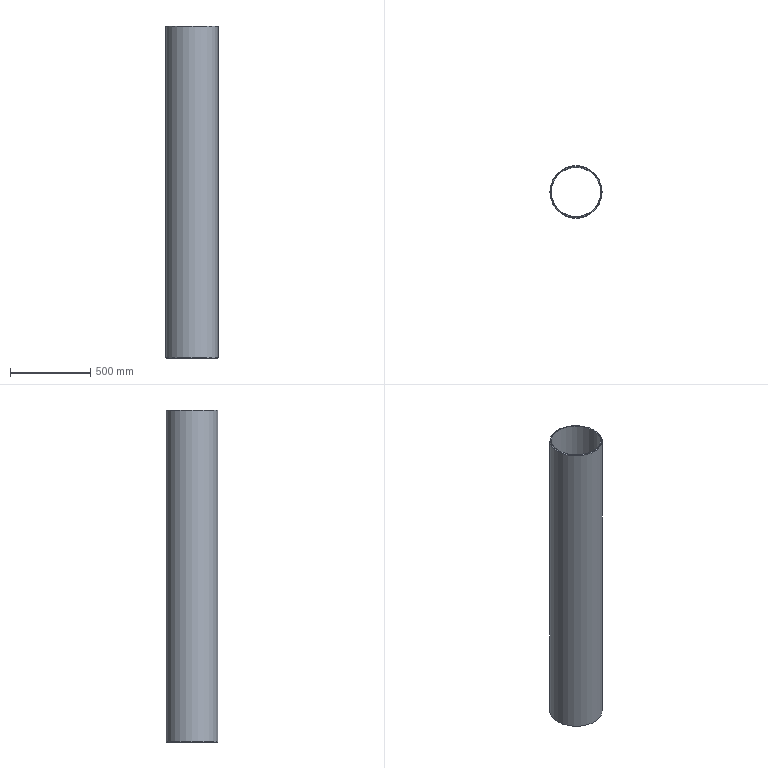Part | NX | features CHAMFER 1, CYLINDER 1, DATUM_CSYS 1, SHELL 1 | 1 solid | 6 faces | box 325 x 325 x 2069 mm | volume 16472932 mm3 | plane 2 | cylinder 2 | cone 2 | commonest cylinder face diameters 309 x1 325 x1
STEP:
#1=CARTESIAN_POINT('',(158.17,0.,2069.));
#2=VERTEX_POINT('',#1);
#3=CARTESIAN_POINT('',(0.,0.,2069.));
#4=DIRECTION('',(0.,0.,1.));
#5=DIRECTION('',(1.,0.,0.));
#6=AXIS2_PLACEMENT_3D('',#3,#4,#5);
#7=CIRCLE('',#6,158.17);
#8=EDGE_CURVE('',#2,#2,#7,.T.);
#9=ORIENTED_EDGE('',*,*,#8,.T.);
#10=EDGE_LOOP('',(#9));
#11=FACE_BOUND('',#10,.T.);
#12=CARTESIAN_POINT('',(154.5,0.,2069.));
#13=VERTEX_POINT('',#12);
#14=CARTESIAN_POINT('',(0.,0.,2069.));
#15=DIRECTION('',(0.,0.,1.));
#16=DIRECTION('',(1.,0.,0.));
#17=AXIS2_PLACEMENT_3D('',#14,#15,#16);
#18=CIRCLE('',#17,154.5);
#19=EDGE_CURVE('',#13,#13,#18,.F.);
#20=ORIENTED_EDGE('',*,*,#19,.T.);
#21=EDGE_LOOP('',(#20));
#22=FACE_BOUND('',#21,.T.);
#23=CARTESIAN_POINT('',(0.,0.,2069.));
#24=DIRECTION('',(0.,0.,1.));
#25=DIRECTION('',(1.,0.,0.));
#26=AXIS2_PLACEMENT_3D('',#23,#24,#25);
#27=PLANE('',#26);
#28=ADVANCED_FACE('',(#11,#22),#27,.T.);
#29=CARTESIAN_POINT('',(-158.17,0.,0.));
#30=VERTEX_POINT('',#29);
#31=CARTESIAN_POINT('',(0.,0.,0.));
#32=DIRECTION('',(0.,0.,-1.));
#33=DIRECTION('',(-1.,0.,0.));
#34=AXIS2_PLACEMENT_3D('',#31,#32,#33);
#35=CIRCLE('',#34,158.17);
#36=EDGE_CURVE('',#30,#30,#35,.T.);
#37=ORIENTED_EDGE('',*,*,#36,.T.);
#38=EDGE_LOOP('',(#37));
#39=FACE_BOUND('',#38,.T.);
#40=CARTESIAN_POINT('',(-154.5,0.,0.));
#41=VERTEX_POINT('',#40);
#42=CARTESIAN_POINT('',(0.,0.,0.));
#43=DIRECTION('',(0.,0.,-1.));
#44=DIRECTION('',(-1.,0.,0.));
#45=AXIS2_PLACEMENT_3D('',#42,#43,#44);
#46=CIRCLE('',#45,154.5);
#47=EDGE_CURVE('',#41,#41,#46,.F.);
#48=ORIENTED_EDGE('',*,*,#47,.T.);
#49=EDGE_LOOP('',(#48));
#50=FACE_BOUND('',#49,.T.);
#51=CARTESIAN_POINT('',(0.,0.,0.));
#52=DIRECTION('',(0.,0.,-1.));
#53=DIRECTION('',(-1.,0.,0.));
#54=AXIS2_PLACEMENT_3D('',#51,#52,#53);
#55=PLANE('',#54);
#56=ADVANCED_FACE('',(#39,#50),#55,.T.);
#57=CARTESIAN_POINT('',(-162.5,0.,2.5));
#58=VERTEX_POINT('',#57);
#59=CARTESIAN_POINT('',(0.,0.,2.5));
#60=DIRECTION('',(0.,0.,-1.));
#61=DIRECTION('',(-1.,0.,0.));
#62=AXIS2_PLACEMENT_3D('',#59,#60,#61);
#63=CIRCLE('',#62,162.5);
#64=EDGE_CURVE('',#58,#58,#63,.F.);
#65=ORIENTED_EDGE('',*,*,#64,.T.);
#66=EDGE_LOOP('',(#65));
#67=FACE_BOUND('',#66,.T.);
#68=CARTESIAN_POINT('',(162.5,0.,2066.5));
#69=VERTEX_POINT('',#68);
#70=CARTESIAN_POINT('',(0.,0.,2066.5));
#71=DIRECTION('',(0.,0.,1.));
#72=DIRECTION('',(1.,0.,0.));
#73=AXIS2_PLACEMENT_3D('',#70,#71,#72);
#74=CIRCLE('',#73,162.5);
#75=EDGE_CURVE('',#69,#69,#74,.F.);
#76=ORIENTED_EDGE('',*,*,#75,.T.);
#77=EDGE_LOOP('',(#76));
#78=FACE_BOUND('',#77,.T.);
#79=CARTESIAN_POINT('',(0.,0.,0.));
#80=DIRECTION('',(0.,0.,1.));
#81=DIRECTION('',(1.,0.,0.));
#82=AXIS2_PLACEMENT_3D('',#79,#80,#81);
#83=CYLINDRICAL_SURFACE('',#82,162.5);
#84=ADVANCED_FACE('',(#67,#78),#83,.T.);
#85=ORIENTED_EDGE('',*,*,#19,.F.);
#86=EDGE_LOOP('',(#85));
#87=FACE_BOUND('',#86,.T.);
#88=ORIENTED_EDGE('',*,*,#47,.F.);
#89=EDGE_LOOP('',(#88));
#90=FACE_BOUND('',#89,.T.);
#91=CARTESIAN_POINT('',(0.,0.,0.));
#92=DIRECTION('',(0.,0.,1.));
#93=DIRECTION('',(1.,0.,0.));
#94=AXIS2_PLACEMENT_3D('',#91,#92,#93);
#95=CYLINDRICAL_SURFACE('',#94,154.5);
#96=ADVANCED_FACE('',(#87,#90),#95,.F.);
#97=ORIENTED_EDGE('',*,*,#36,.F.);
#98=EDGE_LOOP('',(#97));
#99=FACE_BOUND('',#98,.T.);
#100=ORIENTED_EDGE('',*,*,#64,.F.);
#101=EDGE_LOOP('',(#100));
#102=FACE_BOUND('',#101,.T.);
#103=CARTESIAN_POINT('',(0.,0.,2.5));
#104=DIRECTION('',(0.,0.,1.));
#105=DIRECTION('',(1.,0.,0.));
#106=AXIS2_PLACEMENT_3D('',#103,#104,#105);
#107=CONICAL_SURFACE('',#106,162.5,1.047);
#108=ADVANCED_FACE('',(#99,#102),#107,.T.);
#109=ORIENTED_EDGE('',*,*,#8,.F.);
#110=EDGE_LOOP('',(#109));
#111=FACE_BOUND('',#110,.T.);
#112=ORIENTED_EDGE('',*,*,#75,.F.);
#113=EDGE_LOOP('',(#112));
#114=FACE_BOUND('',#113,.T.);
#115=CARTESIAN_POINT('',(0.,0.,2066.5));
#116=DIRECTION('',(0.,0.,-1.));
#117=DIRECTION('',(-1.,0.,0.));
#118=AXIS2_PLACEMENT_3D('',#115,#116,#117);
#119=CONICAL_SURFACE('',#118,162.5,1.047);
#120=ADVANCED_FACE('',(#111,#114),#119,.T.);
#121=CLOSED_SHELL('',(#28,#56,#84,#96,#108,#120));
#122=MANIFOLD_SOLID_BREP('',#121);
#123=(LENGTH_UNIT()NAMED_UNIT(*)SI_UNIT(.MILLI.,.METRE.));
#124=UNCERTAINTY_MEASURE_WITH_UNIT(LENGTH_MEASURE(0.00001),#123,'','');
#125=(NAMED_UNIT(*)PLANE_ANGLE_UNIT()SI_UNIT($,.RADIAN.));
#126=(NAMED_UNIT(*)SI_UNIT($,.STERADIAN.)SOLID_ANGLE_UNIT());
#127=(GEOMETRIC_REPRESENTATION_CONTEXT(3)GLOBAL_UNCERTAINTY_ASSIGNED_CONTEXT((#124))GLOBAL_UNIT_ASSIGNED_CONTEXT((#123,#125,#126))REPRESENTATION_CONTEXT('',''));
#128=ADVANCED_BREP_SHAPE_REPRESENTATION('',(#122),#127);